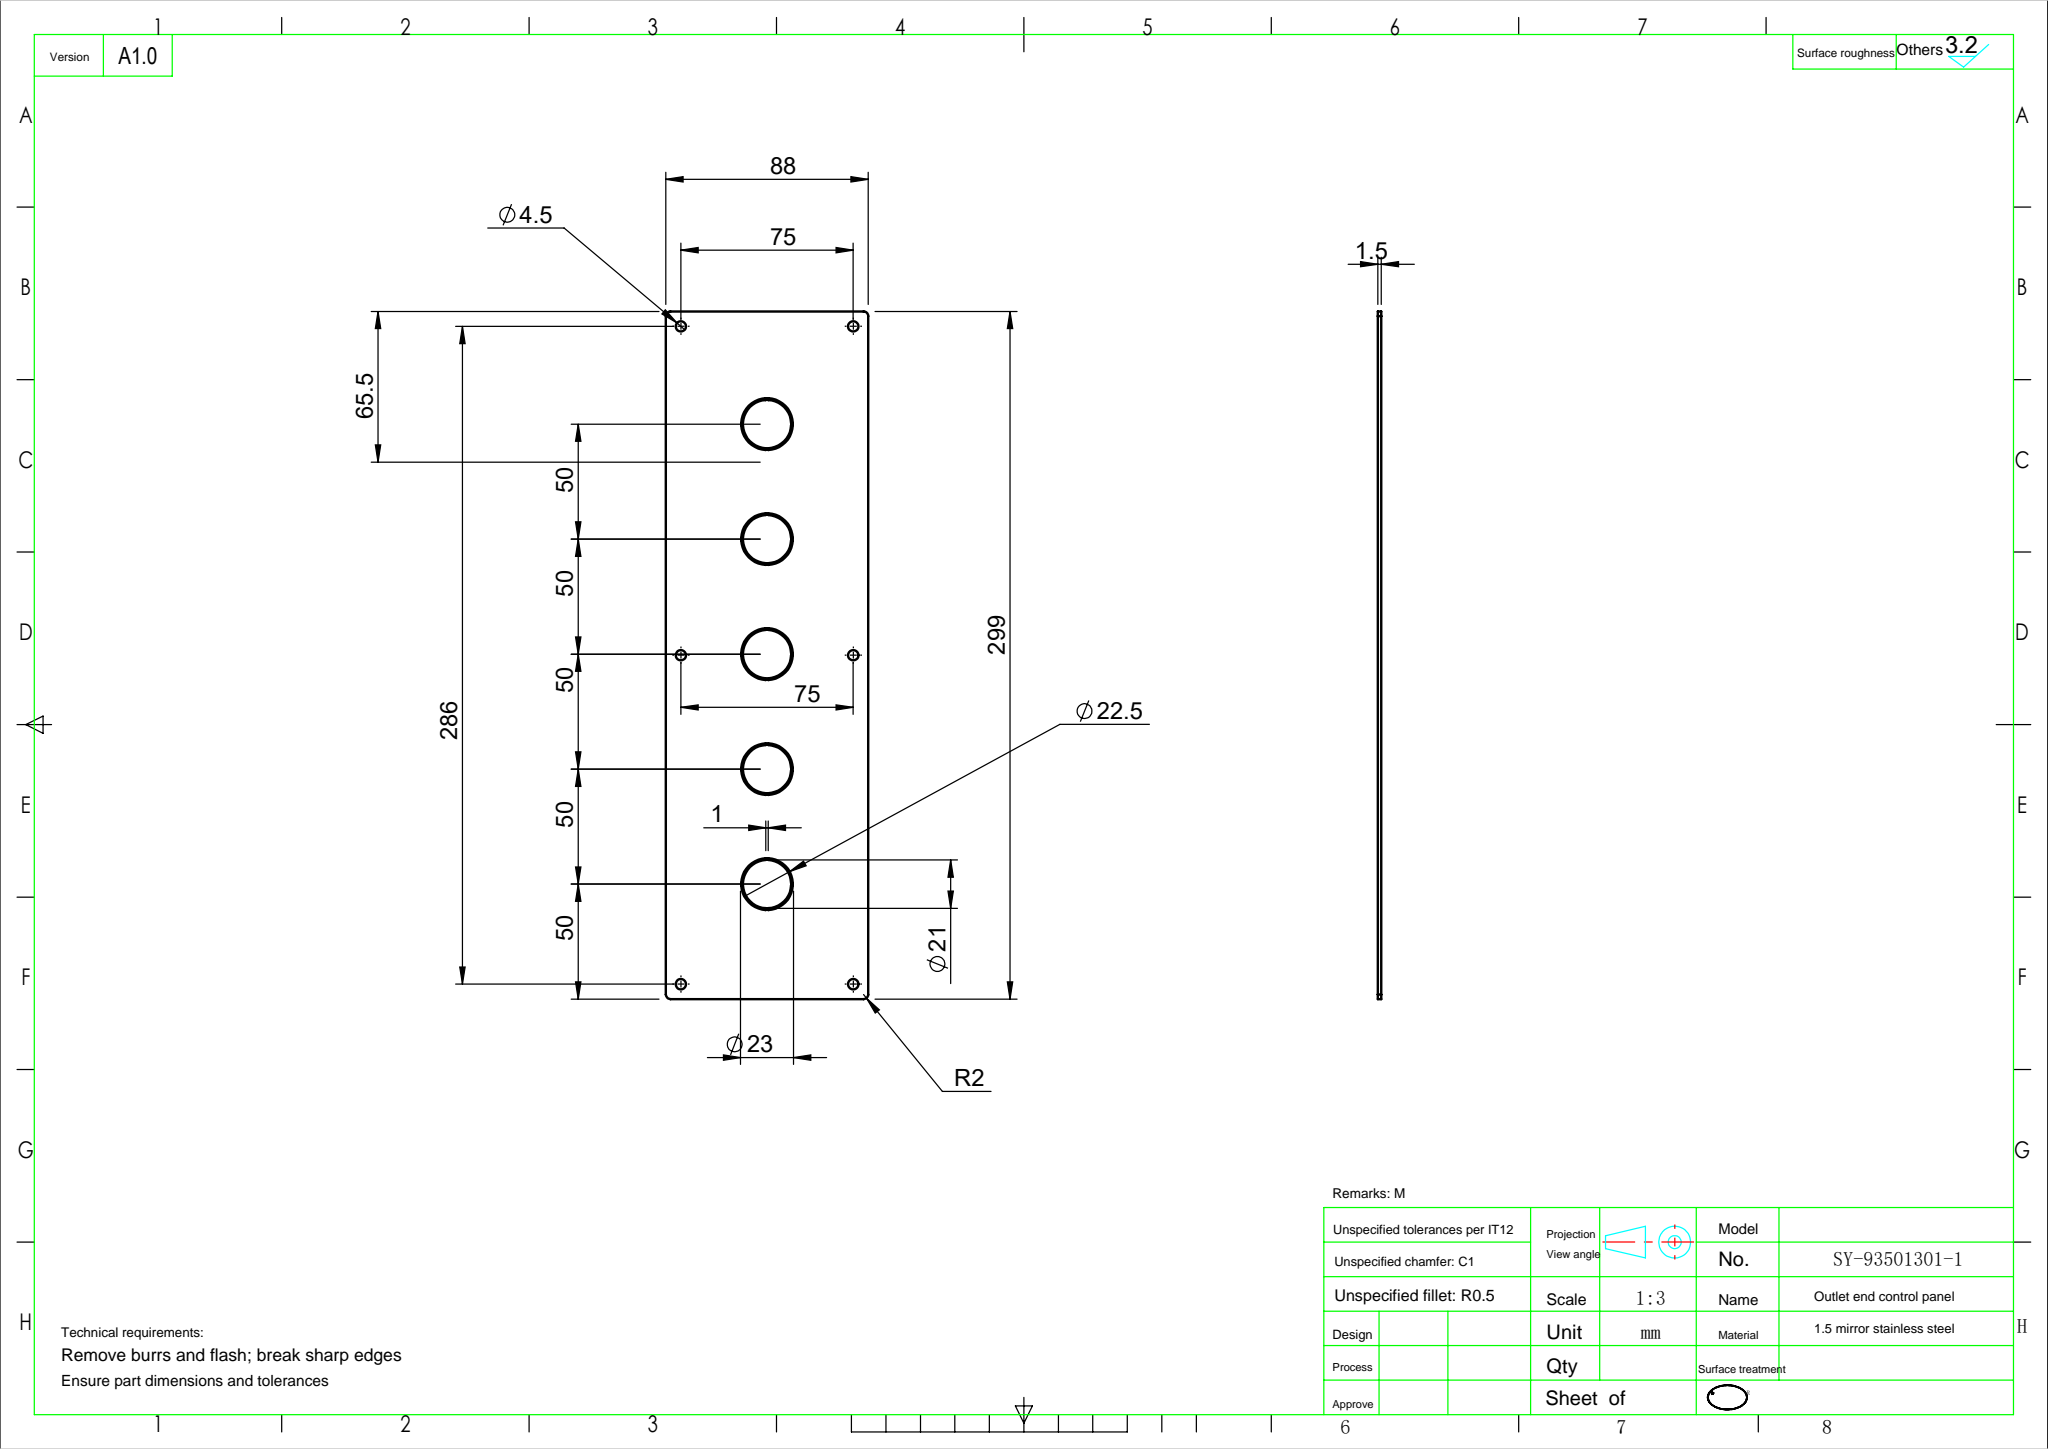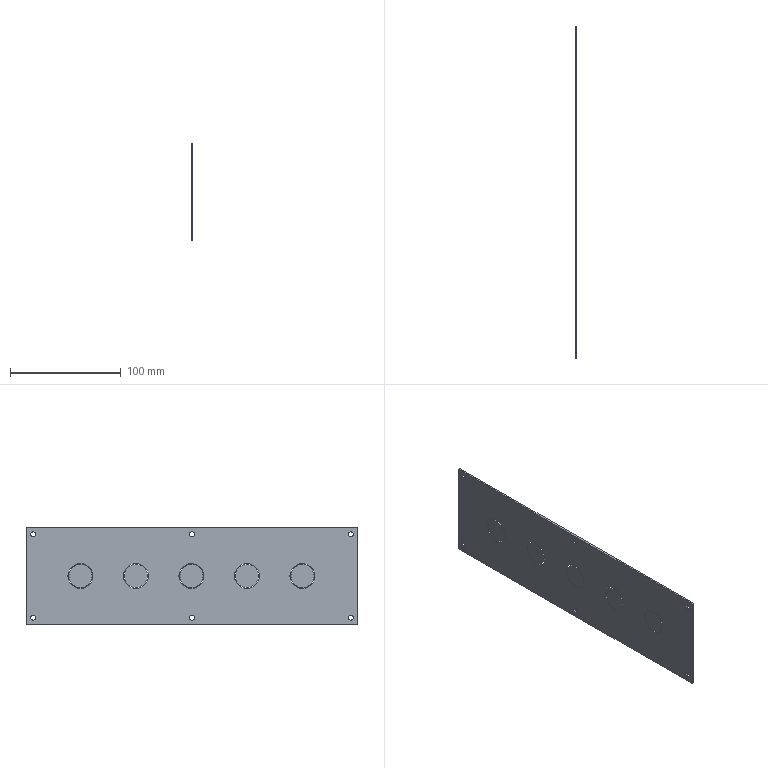Part | SolidWorks | features ICE 2, SMBaseFlange 2, Fillet 1, FlatPattern 1, LPattern 1, SheetMetal 1 | 1 solid | 102 faces | box 1.5 x 299 x 88 mm | volume 38958 mm3 | cylinder 56 | plane 46 | commonest cylinder face diameters 21 x20 22.5 x20 4.5 x12 4 x4